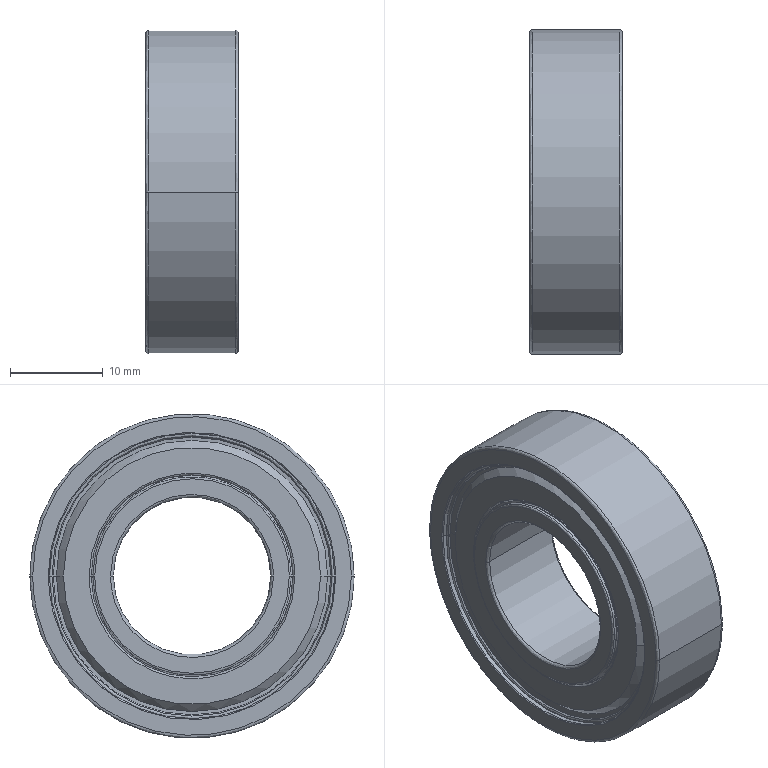Part | SolidWorks | features BaseBody 1 | 1 solid | 136 faces | box 10 x 35 x 35 mm | volume 5865 mm3 | spline 52 | cone 40 | cylinder 32 | plane 12 | commonest cylinder face diameters 20.6 x4 21.4 x4 21.8 x4 22.2 x4 22.6 x4 29.4 x4